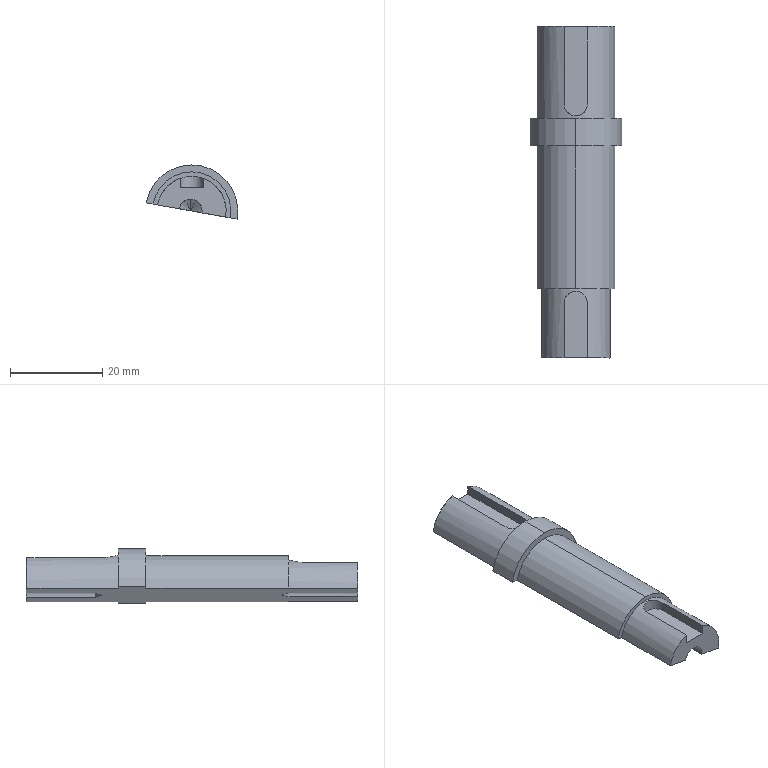Part | STEP file | Cuon T phu H01_2 | 1 solid | 29 faces | box 19.843 x 72 x 11.76 mm | volume 7356 mm3 | plane 12 | cylinder 11 | cone 6 | commonest cylinder face diameters 5 x5 17 x3 20 x2 15 x1